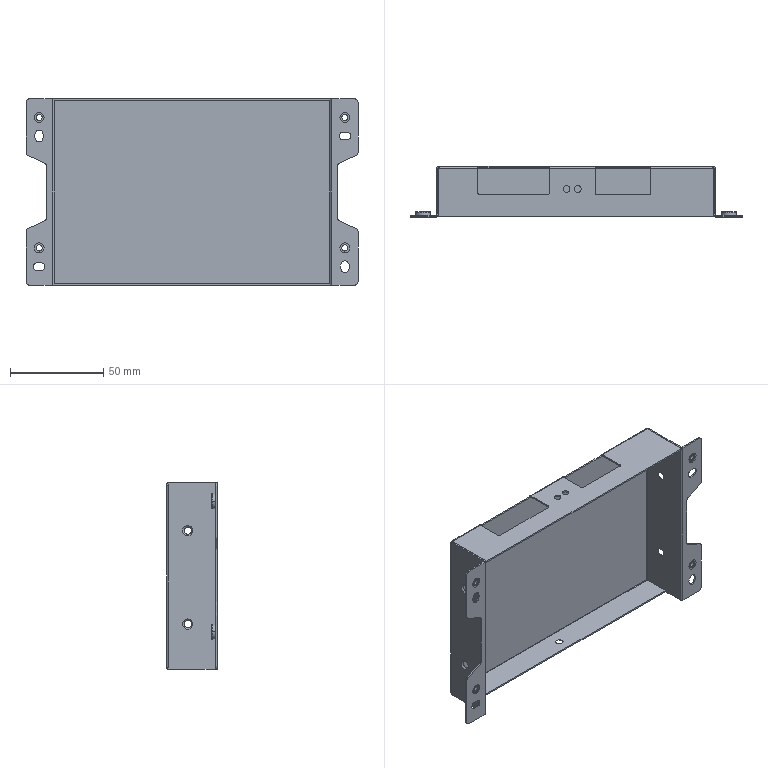Part | SolidWorks | features BaseBody 5, ICE 2 | 5 solids | 172 faces | box 177.9 x 27.2 x 100 mm | volume 21775 mm3 | cylinder 84 | plane 66 | spline 12 | cone 10 | commonest cylinder face diameters 4 x20 2 x12 4.2 x10 0.4 x8 3.3 x8 5.4 x8